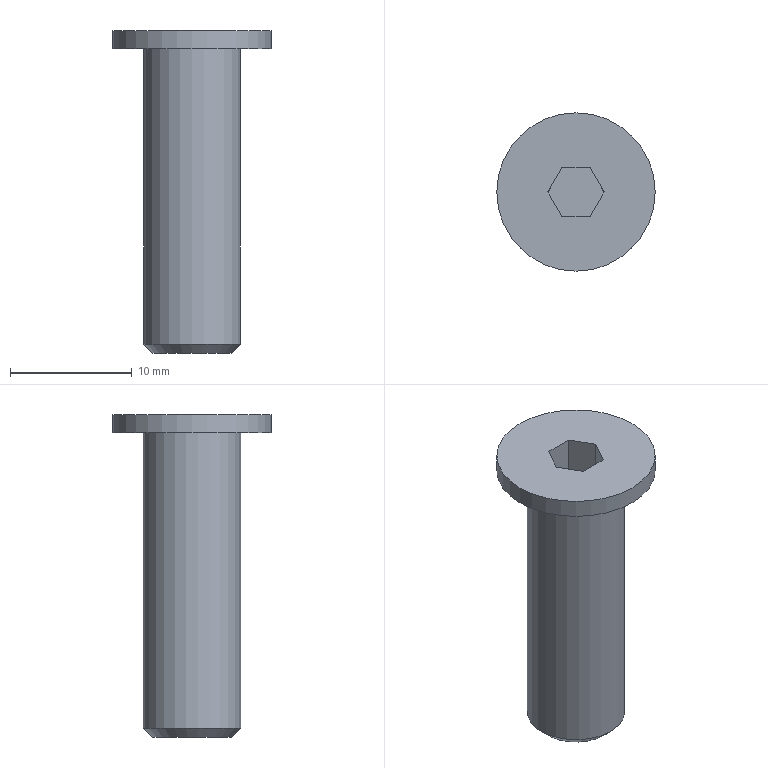Part | STEP file | 1 solid | 13 faces | box 13 x 13 x 26.5 mm | volume 1380 mm3 | plane 10 | cylinder 2 | cone 1 | commonest cylinder face diameters 8 x1 13 x1
STEP:
#1=CARTESIAN_POINT('',(0.,0.,0.));
#2=DIRECTION('',(0.,0.,1.));
#3=DIRECTION('',(1.,0.,0.));
#4=AXIS2_PLACEMENT_3D('',#1,#2,#3);
#5=CARTESIAN_POINT('',(0.,-6.5,26.5));
#6=VERTEX_POINT('',#5);
#7=CARTESIAN_POINT('',(0.,0.,26.5));
#8=DIRECTION('',(0.,0.,1.));
#9=DIRECTION('',(1.,0.,0.));
#10=AXIS2_PLACEMENT_3D('',#7,#8,#9);
#11=CIRCLE('',#10,6.5);
#12=CARTESIAN_POINT('',(0.,0.,25.75));
#13=DIRECTION('',(0.,0.,1.));
#14=DIRECTION('',(0.,1.,0.));
#15=AXIS2_PLACEMENT_3D('',#12,#13,#14);
#16=CYLINDRICAL_SURFACE('',#15,6.5);
#17=CARTESIAN_POINT('',(-1.571,0.75));
#18=DIRECTION('',(1.,0.));
#19=VECTOR('',#18,1.);
#20=LINE('',#17,#19);
#21=(GEOMETRIC_REPRESENTATION_CONTEXT(2)PARAMETRIC_REPRESENTATION_CONTEXT()REPRESENTATION_CONTEXT('',''));
#22=DEFINITIONAL_REPRESENTATION('',(#20),#21);
#23=PCURVE('',#16,#22);
#24=CARTESIAN_POINT('',(0.,3.25,26.5));
#25=DIRECTION('',(0.,0.,-1.));
#26=DIRECTION('',(-1.,0.,0.));
#27=AXIS2_PLACEMENT_3D('',#24,#25,#26);
#28=PLANE('',#27);
#29=CARTESIAN_POINT('',(-6.5,-3.25));
#30=CARTESIAN_POINT('',(-6.5,8.008));
#31=CARTESIAN_POINT('',(3.25,2.379));
#32=CARTESIAN_POINT('',(13.,-3.25));
#33=CARTESIAN_POINT('',(3.25,-8.879));
#34=CARTESIAN_POINT('',(-6.5,-14.508));
#35=CARTESIAN_POINT('',(-6.5,-3.25));
#36=(BOUNDED_CURVE()B_SPLINE_CURVE(2,(#29,#30,#31,#32,#33,#34,#35),.UNSPECIFIED.,.T.,.F.)B_SPLINE_CURVE_WITH_KNOTS((1,2,2,2,2,1),(-2.094,0.,2.094,4.189,6.283,8.378),.UNSPECIFIED.)CURVE()GEOMETRIC_REPRESENTATION_ITEM()RATIONAL_B_SPLINE_CURVE((1.,0.5,1.,0.5,1.,0.5,1.))REPRESENTATION_ITEM(''));
#37=(GEOMETRIC_REPRESENTATION_CONTEXT(2)PARAMETRIC_REPRESENTATION_CONTEXT()REPRESENTATION_CONTEXT('',''));
#38=DEFINITIONAL_REPRESENTATION('',(#36),#37);
#39=PCURVE('',#28,#38);
#40=SURFACE_CURVE('',#11,(#23,#39),.PCURVE_S1.);
#41=EDGE_CURVE('',#6,#6,#40,.T.);
#42=ORIENTED_EDGE('',*,*,#41,.F.);
#43=CARTESIAN_POINT('',(0.,-6.5,25.));
#44=VERTEX_POINT('',#43);
#45=CARTESIAN_POINT('',(0.,-6.5,25.));
#46=CARTESIAN_POINT('',(0.,-6.5,26.5));
#47=B_SPLINE_CURVE_WITH_KNOTS('',1,(#45,#46),.UNSPECIFIED.,.F.,.F.,(2,2),(-0.75,0.75),.PIECEWISE_BEZIER_KNOTS.);
#48=CARTESIAN_POINT('',(3.142,0.));
#49=DIRECTION('',(0.,1.));
#50=VECTOR('',#49,1.);
#51=LINE('',#48,#50);
#52=(GEOMETRIC_REPRESENTATION_CONTEXT(2)PARAMETRIC_REPRESENTATION_CONTEXT()REPRESENTATION_CONTEXT('',''));
#53=DEFINITIONAL_REPRESENTATION('',(#51),#52);
#54=PCURVE('',#16,#53);
#55=CARTESIAN_POINT('',(9.425,0.));
#56=DIRECTION('',(0.,1.));
#57=VECTOR('',#56,1.);
#58=LINE('',#55,#57);
#59=(GEOMETRIC_REPRESENTATION_CONTEXT(2)PARAMETRIC_REPRESENTATION_CONTEXT()REPRESENTATION_CONTEXT('',''));
#60=DEFINITIONAL_REPRESENTATION('',(#58),#59);
#61=PCURVE('',#16,#60);
#62=SEAM_CURVE('',#47,(#54,#61),.PCURVE_S1.);
#63=EDGE_CURVE('',#44,#6,#62,.T.);
#64=ORIENTED_EDGE('',*,*,#63,.F.);
#65=CARTESIAN_POINT('',(0.,0.,25.));
#66=DIRECTION('',(0.,0.,1.));
#67=DIRECTION('',(1.,0.,0.));
#68=AXIS2_PLACEMENT_3D('',#65,#66,#67);
#69=CIRCLE('',#68,6.5);
#70=CARTESIAN_POINT('',(-1.571,-0.75));
#71=DIRECTION('',(1.,0.));
#72=VECTOR('',#71,1.);
#73=LINE('',#70,#72);
#74=(GEOMETRIC_REPRESENTATION_CONTEXT(2)PARAMETRIC_REPRESENTATION_CONTEXT()REPRESENTATION_CONTEXT('',''));
#75=DEFINITIONAL_REPRESENTATION('',(#73),#74);
#76=PCURVE('',#16,#75);
#77=CARTESIAN_POINT('',(0.,5.25,25.));
#78=DIRECTION('',(0.,0.,-1.));
#79=DIRECTION('',(-1.,0.,0.));
#80=AXIS2_PLACEMENT_3D('',#77,#78,#79);
#81=PLANE('',#80);
#82=CARTESIAN_POINT('',(-6.5,-5.25));
#83=CARTESIAN_POINT('',(-6.5,6.008));
#84=CARTESIAN_POINT('',(3.25,0.3792));
#85=CARTESIAN_POINT('',(13.,-5.25));
#86=CARTESIAN_POINT('',(3.25,-10.879));
#87=CARTESIAN_POINT('',(-6.5,-16.508));
#88=CARTESIAN_POINT('',(-6.5,-5.25));
#89=(BOUNDED_CURVE()B_SPLINE_CURVE(2,(#82,#83,#84,#85,#86,#87,#88),.UNSPECIFIED.,.T.,.F.)B_SPLINE_CURVE_WITH_KNOTS((1,2,2,2,2,1),(-2.094,0.,2.094,4.189,6.283,8.378),.UNSPECIFIED.)CURVE()GEOMETRIC_REPRESENTATION_ITEM()RATIONAL_B_SPLINE_CURVE((1.,0.5,1.,0.5,1.,0.5,1.))REPRESENTATION_ITEM(''));
#90=(GEOMETRIC_REPRESENTATION_CONTEXT(2)PARAMETRIC_REPRESENTATION_CONTEXT()REPRESENTATION_CONTEXT('',''));
#91=DEFINITIONAL_REPRESENTATION('',(#89),#90);
#92=PCURVE('',#81,#91);
#93=SURFACE_CURVE('',#69,(#76,#92),.PCURVE_S1.);
#94=EDGE_CURVE('',#44,#44,#93,.T.);
#95=ORIENTED_EDGE('',*,*,#94,.T.);
#96=ORIENTED_EDGE('',*,*,#63,.T.);
#97=EDGE_LOOP('',(#42,#64,#95,#96));
#98=FACE_BOUND('',#97,.T.);
#99=ADVANCED_FACE('',(#98),#16,.T.);
#100=ORIENTED_EDGE('',*,*,#41,.T.);
#101=EDGE_LOOP('',(#100));
#102=FACE_BOUND('',#101,.T.);
#103=CARTESIAN_POINT('',(-2.309,0.,26.5));
#104=VERTEX_POINT('',#103);
#105=CARTESIAN_POINT('',(-1.155,2.,26.5));
#106=VERTEX_POINT('',#105);
#107=CARTESIAN_POINT('',(-2.309,0.,26.5));
#108=DIRECTION('',(0.5,0.866,0.));
#109=VECTOR('',#108,1.);
#110=LINE('',#107,#109);
#111=CARTESIAN_POINT('',(2.309,-3.25));
#112=DIRECTION('',(-0.5,0.866));
#113=VECTOR('',#112,1.);
#114=LINE('',#111,#113);
#115=(GEOMETRIC_REPRESENTATION_CONTEXT(2)PARAMETRIC_REPRESENTATION_CONTEXT()REPRESENTATION_CONTEXT('',''));
#116=DEFINITIONAL_REPRESENTATION('',(#114),#115);
#117=PCURVE('',#28,#116);
#118=CARTESIAN_POINT('',(-1.155,2.,26.5));
#119=DIRECTION('',(-0.866,0.5,0.));
#120=DIRECTION('',(0.,0.,1.));
#121=AXIS2_PLACEMENT_3D('',#118,#119,#120);
#122=PLANE('',#121);
#123=CARTESIAN_POINT('',(0.,-2.309));
#124=DIRECTION('',(0.,1.));
#125=VECTOR('',#124,1.);
#126=LINE('',#123,#125);
#127=(GEOMETRIC_REPRESENTATION_CONTEXT(2)PARAMETRIC_REPRESENTATION_CONTEXT()REPRESENTATION_CONTEXT('',''));
#128=DEFINITIONAL_REPRESENTATION('',(#126),#127);
#129=PCURVE('',#122,#128);
#130=SURFACE_CURVE('',#110,(#117,#129),.PCURVE_S1.);
#131=EDGE_CURVE('',#104,#106,#130,.T.);
#132=ORIENTED_EDGE('',*,*,#131,.T.);
#133=CARTESIAN_POINT('',(1.155,2.,26.5));
#134=VERTEX_POINT('',#133);
#135=CARTESIAN_POINT('',(-1.155,2.,26.5));
#136=DIRECTION('',(1.,0.,0.));
#137=VECTOR('',#136,1.);
#138=LINE('',#135,#137);
#139=CARTESIAN_POINT('',(1.155,-1.25));
#140=DIRECTION('',(-1.,0.));
#141=VECTOR('',#140,1.);
#142=LINE('',#139,#141);
#143=(GEOMETRIC_REPRESENTATION_CONTEXT(2)PARAMETRIC_REPRESENTATION_CONTEXT()REPRESENTATION_CONTEXT('',''));
#144=DEFINITIONAL_REPRESENTATION('',(#142),#143);
#145=PCURVE('',#28,#144);
#146=CARTESIAN_POINT('',(1.155,2.,26.5));
#147=DIRECTION('',(0.,1.,0.));
#148=DIRECTION('',(0.,0.,1.));
#149=AXIS2_PLACEMENT_3D('',#146,#147,#148);
#150=PLANE('',#149);
#151=CARTESIAN_POINT('',(0.,-2.309));
#152=DIRECTION('',(0.,1.));
#153=VECTOR('',#152,1.);
#154=LINE('',#151,#153);
#155=(GEOMETRIC_REPRESENTATION_CONTEXT(2)PARAMETRIC_REPRESENTATION_CONTEXT()REPRESENTATION_CONTEXT('',''));
#156=DEFINITIONAL_REPRESENTATION('',(#154),#155);
#157=PCURVE('',#150,#156);
#158=SURFACE_CURVE('',#138,(#145,#157),.PCURVE_S1.);
#159=EDGE_CURVE('',#106,#134,#158,.T.);
#160=ORIENTED_EDGE('',*,*,#159,.T.);
#161=CARTESIAN_POINT('',(2.309,0.,26.5));
#162=VERTEX_POINT('',#161);
#163=CARTESIAN_POINT('',(1.155,2.,26.5));
#164=DIRECTION('',(0.5,-0.866,0.));
#165=VECTOR('',#164,1.);
#166=LINE('',#163,#165);
#167=CARTESIAN_POINT('',(-1.155,-1.25));
#168=DIRECTION('',(-0.5,-0.866));
#169=VECTOR('',#168,1.);
#170=LINE('',#167,#169);
#171=(GEOMETRIC_REPRESENTATION_CONTEXT(2)PARAMETRIC_REPRESENTATION_CONTEXT()REPRESENTATION_CONTEXT('',''));
#172=DEFINITIONAL_REPRESENTATION('',(#170),#171);
#173=PCURVE('',#28,#172);
#174=CARTESIAN_POINT('',(2.309,0.,26.5));
#175=DIRECTION('',(0.866,0.5,0.));
#176=DIRECTION('',(0.,0.,-1.));
#177=AXIS2_PLACEMENT_3D('',#174,#175,#176);
#178=PLANE('',#177);
#179=CARTESIAN_POINT('',(0.,2.309));
#180=DIRECTION('',(0.,-1.));
#181=VECTOR('',#180,1.);
#182=LINE('',#179,#181);
#183=(GEOMETRIC_REPRESENTATION_CONTEXT(2)PARAMETRIC_REPRESENTATION_CONTEXT()REPRESENTATION_CONTEXT('',''));
#184=DEFINITIONAL_REPRESENTATION('',(#182),#183);
#185=PCURVE('',#178,#184);
#186=SURFACE_CURVE('',#166,(#173,#185),.PCURVE_S1.);
#187=EDGE_CURVE('',#134,#162,#186,.T.);
#188=ORIENTED_EDGE('',*,*,#187,.T.);
#189=CARTESIAN_POINT('',(1.155,-2.,26.5));
#190=VERTEX_POINT('',#189);
#191=CARTESIAN_POINT('',(2.309,0.,26.5));
#192=DIRECTION('',(-0.5,-0.866,0.));
#193=VECTOR('',#192,1.);
#194=LINE('',#191,#193);
#195=CARTESIAN_POINT('',(-2.309,-3.25));
#196=DIRECTION('',(0.5,-0.866));
#197=VECTOR('',#196,1.);
#198=LINE('',#195,#197);
#199=(GEOMETRIC_REPRESENTATION_CONTEXT(2)PARAMETRIC_REPRESENTATION_CONTEXT()REPRESENTATION_CONTEXT('',''));
#200=DEFINITIONAL_REPRESENTATION('',(#198),#199);
#201=PCURVE('',#28,#200);
#202=CARTESIAN_POINT('',(1.155,-2.,26.5));
#203=DIRECTION('',(0.866,-0.5,0.));
#204=DIRECTION('',(0.,0.,-1.));
#205=AXIS2_PLACEMENT_3D('',#202,#203,#204);
#206=PLANE('',#205);
#207=CARTESIAN_POINT('',(0.,2.309));
#208=DIRECTION('',(0.,-1.));
#209=VECTOR('',#208,1.);
#210=LINE('',#207,#209);
#211=(GEOMETRIC_REPRESENTATION_CONTEXT(2)PARAMETRIC_REPRESENTATION_CONTEXT()REPRESENTATION_CONTEXT('',''));
#212=DEFINITIONAL_REPRESENTATION('',(#210),#211);
#213=PCURVE('',#206,#212);
#214=SURFACE_CURVE('',#194,(#201,#213),.PCURVE_S1.);
#215=EDGE_CURVE('',#162,#190,#214,.T.);
#216=ORIENTED_EDGE('',*,*,#215,.T.);
#217=CARTESIAN_POINT('',(-1.155,-2.,26.5));
#218=VERTEX_POINT('',#217);
#219=CARTESIAN_POINT('',(1.155,-2.,26.5));
#220=DIRECTION('',(-1.,0.,0.));
#221=VECTOR('',#220,1.);
#222=LINE('',#219,#221);
#223=CARTESIAN_POINT('',(-1.155,-5.25));
#224=DIRECTION('',(1.,0.));
#225=VECTOR('',#224,1.);
#226=LINE('',#223,#225);
#227=(GEOMETRIC_REPRESENTATION_CONTEXT(2)PARAMETRIC_REPRESENTATION_CONTEXT()REPRESENTATION_CONTEXT('',''));
#228=DEFINITIONAL_REPRESENTATION('',(#226),#227);
#229=PCURVE('',#28,#228);
#230=CARTESIAN_POINT('',(-1.155,-2.,26.5));
#231=DIRECTION('',(0.,-1.,0.));
#232=DIRECTION('',(0.,0.,-1.));
#233=AXIS2_PLACEMENT_3D('',#230,#231,#232);
#234=PLANE('',#233);
#235=CARTESIAN_POINT('',(0.,2.309));
#236=DIRECTION('',(0.,-1.));
#237=VECTOR('',#236,1.);
#238=LINE('',#235,#237);
#239=(GEOMETRIC_REPRESENTATION_CONTEXT(2)PARAMETRIC_REPRESENTATION_CONTEXT()REPRESENTATION_CONTEXT('',''));
#240=DEFINITIONAL_REPRESENTATION('',(#238),#239);
#241=PCURVE('',#234,#240);
#242=SURFACE_CURVE('',#222,(#229,#241),.PCURVE_S1.);
#243=EDGE_CURVE('',#190,#218,#242,.T.);
#244=ORIENTED_EDGE('',*,*,#243,.T.);
#245=CARTESIAN_POINT('',(-1.155,-2.,26.5));
#246=DIRECTION('',(-0.5,0.866,0.));
#247=VECTOR('',#246,1.);
#248=LINE('',#245,#247);
#249=CARTESIAN_POINT('',(1.155,-5.25));
#250=DIRECTION('',(0.5,0.866));
#251=VECTOR('',#250,1.);
#252=LINE('',#249,#251);
#253=(GEOMETRIC_REPRESENTATION_CONTEXT(2)PARAMETRIC_REPRESENTATION_CONTEXT()REPRESENTATION_CONTEXT('',''));
#254=DEFINITIONAL_REPRESENTATION('',(#252),#253);
#255=PCURVE('',#28,#254);
#256=CARTESIAN_POINT('',(-2.309,0.,26.5));
#257=DIRECTION('',(-0.866,-0.5,0.));
#258=DIRECTION('',(0.,0.,1.));
#259=AXIS2_PLACEMENT_3D('',#256,#257,#258);
#260=PLANE('',#259);
#261=CARTESIAN_POINT('',(0.,-2.309));
#262=DIRECTION('',(0.,1.));
#263=VECTOR('',#262,1.);
#264=LINE('',#261,#263);
#265=(GEOMETRIC_REPRESENTATION_CONTEXT(2)PARAMETRIC_REPRESENTATION_CONTEXT()REPRESENTATION_CONTEXT('',''));
#266=DEFINITIONAL_REPRESENTATION('',(#264),#265);
#267=PCURVE('',#260,#266);
#268=SURFACE_CURVE('',#248,(#255,#267),.PCURVE_S1.);
#269=EDGE_CURVE('',#218,#104,#268,.T.);
#270=ORIENTED_EDGE('',*,*,#269,.T.);
#271=EDGE_LOOP('',(#132,#160,#188,#216,#244,#270));
#272=FACE_BOUND('',#271,.T.);
#273=ADVANCED_FACE('',(#102,#272),#28,.F.);
#274=ORIENTED_EDGE('',*,*,#94,.F.);
#275=EDGE_LOOP('',(#274));
#276=FACE_BOUND('',#275,.T.);
#277=CARTESIAN_POINT('',(0.,-4.,25.));
#278=VERTEX_POINT('',#277);
#279=CARTESIAN_POINT('',(0.,0.,25.));
#280=DIRECTION('',(0.,0.,-1.));
#281=DIRECTION('',(1.,0.,0.));
#282=AXIS2_PLACEMENT_3D('',#279,#280,#281);
#283=CIRCLE('',#282,4.);
#284=CARTESIAN_POINT('',(0.,-5.25));
#285=DIRECTION('',(-1.,0.));
#286=AXIS2_PLACEMENT_2D('',#284,#285);
#287=CIRCLE('',#286,4.);
#288=(GEOMETRIC_REPRESENTATION_CONTEXT(2)PARAMETRIC_REPRESENTATION_CONTEXT()REPRESENTATION_CONTEXT('',''));
#289=DEFINITIONAL_REPRESENTATION('',(#287),#288);
#290=PCURVE('',#81,#289);
#291=CARTESIAN_POINT('',(0.,0.,12.883));
#292=DIRECTION('',(0.,0.,1.));
#293=DIRECTION('',(0.,1.,0.));
#294=AXIS2_PLACEMENT_3D('',#291,#292,#293);
#295=CYLINDRICAL_SURFACE('',#294,4.);
#296=CARTESIAN_POINT('',(10.996,12.117));
#297=DIRECTION('',(-1.,0.));
#298=VECTOR('',#297,1.);
#299=LINE('',#296,#298);
#300=(GEOMETRIC_REPRESENTATION_CONTEXT(2)PARAMETRIC_REPRESENTATION_CONTEXT()REPRESENTATION_CONTEXT('',''));
#301=DEFINITIONAL_REPRESENTATION('',(#299),#300);
#302=PCURVE('',#295,#301);
#303=SURFACE_CURVE('',#283,(#290,#302),.PCURVE_S1.);
#304=EDGE_CURVE('',#278,#278,#303,.T.);
#305=ORIENTED_EDGE('',*,*,#304,.F.);
#306=EDGE_LOOP('',(#305));
#307=FACE_BOUND('',#306,.T.);
#308=ADVANCED_FACE('',(#276,#307),#81,.T.);
#309=CARTESIAN_POINT('',(-2.309,0.,21.5));
#310=VERTEX_POINT('',#309);
#311=CARTESIAN_POINT('',(-2.309,0.,26.5));
#312=DIRECTION('',(0.,0.,-1.));
#313=VECTOR('',#312,1.);
#314=LINE('',#311,#313);
#315=CARTESIAN_POINT('',(0.,-2.309));
#316=DIRECTION('',(-1.,0.));
#317=VECTOR('',#316,1.);
#318=LINE('',#315,#317);
#319=(GEOMETRIC_REPRESENTATION_CONTEXT(2)PARAMETRIC_REPRESENTATION_CONTEXT()REPRESENTATION_CONTEXT('',''));
#320=DEFINITIONAL_REPRESENTATION('',(#318),#319);
#321=PCURVE('',#122,#320);
#322=CARTESIAN_POINT('',(0.,0.));
#323=DIRECTION('',(-1.,0.));
#324=VECTOR('',#323,1.);
#325=LINE('',#322,#324);
#326=(GEOMETRIC_REPRESENTATION_CONTEXT(2)PARAMETRIC_REPRESENTATION_CONTEXT()REPRESENTATION_CONTEXT('',''));
#327=DEFINITIONAL_REPRESENTATION('',(#325),#326);
#328=PCURVE('',#260,#327);
#329=SURFACE_CURVE('',#314,(#321,#328),.PCURVE_S1.);
#330=EDGE_CURVE('',#104,#310,#329,.T.);
#331=ORIENTED_EDGE('',*,*,#330,.T.);
#332=CARTESIAN_POINT('',(-1.155,2.,21.5));
#333=VERTEX_POINT('',#332);
#334=CARTESIAN_POINT('',(-1.155,2.,21.5));
#335=DIRECTION('',(-0.5,-0.866,0.));
#336=VECTOR('',#335,1.);
#337=LINE('',#334,#336);
#338=CARTESIAN_POINT('',(-5.,0.));
#339=DIRECTION('',(0.,-1.));
#340=VECTOR('',#339,1.);
#341=LINE('',#338,#340);
#342=(GEOMETRIC_REPRESENTATION_CONTEXT(2)PARAMETRIC_REPRESENTATION_CONTEXT()REPRESENTATION_CONTEXT('',''));
#343=DEFINITIONAL_REPRESENTATION('',(#341),#342);
#344=PCURVE('',#122,#343);
#345=CARTESIAN_POINT('',(0.,0.,21.5));
#346=DIRECTION('',(0.,0.,1.));
#347=DIRECTION('',(1.,0.,0.));
#348=AXIS2_PLACEMENT_3D('',#345,#346,#347);
#349=PLANE('',#348);
#350=CARTESIAN_POINT('',(-1.155,2.));
#351=DIRECTION('',(-0.5,-0.866));
#352=VECTOR('',#351,1.);
#353=LINE('',#350,#352);
#354=(GEOMETRIC_REPRESENTATION_CONTEXT(2)PARAMETRIC_REPRESENTATION_CONTEXT()REPRESENTATION_CONTEXT('',''));
#355=DEFINITIONAL_REPRESENTATION('',(#353),#354);
#356=PCURVE('',#349,#355);
#357=SURFACE_CURVE('',#337,(#344,#356),.PCURVE_S1.);
#358=EDGE_CURVE('',#333,#310,#357,.T.);
#359=ORIENTED_EDGE('',*,*,#358,.F.);
#360=CARTESIAN_POINT('',(-1.155,2.,26.5));
#361=DIRECTION('',(0.,0.,-1.));
#362=VECTOR('',#361,1.);
#363=LINE('',#360,#362);
#364=CARTESIAN_POINT('',(0.,0.));
#365=DIRECTION('',(-1.,0.));
#366=VECTOR('',#365,1.);
#367=LINE('',#364,#366);
#368=(GEOMETRIC_REPRESENTATION_CONTEXT(2)PARAMETRIC_REPRESENTATION_CONTEXT()REPRESENTATION_CONTEXT('',''));
#369=DEFINITIONAL_REPRESENTATION('',(#367),#368);
#370=PCURVE('',#122,#369);
#371=CARTESIAN_POINT('',(0.,-2.309));
#372=DIRECTION('',(-1.,0.));
#373=VECTOR('',#372,1.);
#374=LINE('',#371,#373);
#375=(GEOMETRIC_REPRESENTATION_CONTEXT(2)PARAMETRIC_REPRESENTATION_CONTEXT()REPRESENTATION_CONTEXT('',''));
#376=DEFINITIONAL_REPRESENTATION('',(#374),#375);
#377=PCURVE('',#150,#376);
#378=SURFACE_CURVE('',#363,(#370,#377),.PCURVE_S1.);
#379=EDGE_CURVE('',#106,#333,#378,.T.);
#380=ORIENTED_EDGE('',*,*,#379,.F.);
#381=ORIENTED_EDGE('',*,*,#131,.F.);
#382=EDGE_LOOP('',(#331,#359,#380,#381));
#383=FACE_BOUND('',#382,.T.);
#384=ADVANCED_FACE('',(#383),#122,.F.);
#385=ORIENTED_EDGE('',*,*,#379,.T.);
#386=CARTESIAN_POINT('',(1.155,2.,21.5));
#387=VERTEX_POINT('',#386);
#388=CARTESIAN_POINT('',(1.155,2.,21.5));
#389=DIRECTION('',(-1.,0.,0.));
#390=VECTOR('',#389,1.);
#391=LINE('',#388,#390);
#392=CARTESIAN_POINT('',(-5.,0.));
#393=DIRECTION('',(0.,-1.));
#394=VECTOR('',#393,1.);
#395=LINE('',#392,#394);
#396=(GEOMETRIC_REPRESENTATION_CONTEXT(2)PARAMETRIC_REPRESENTATION_CONTEXT()REPRESENTATION_CONTEXT('',''));
#397=DEFINITIONAL_REPRESENTATION('',(#395),#396);
#398=PCURVE('',#150,#397);
#399=CARTESIAN_POINT('',(1.155,2.));
#400=DIRECTION('',(-1.,0.));
#401=VECTOR('',#400,1.);
#402=LINE('',#399,#401);
#403=(GEOMETRIC_REPRESENTATION_CONTEXT(2)PARAMETRIC_REPRESENTATION_CONTEXT()REPRESENTATION_CONTEXT('',''));
#404=DEFINITIONAL_REPRESENTATION('',(#402),#403);
#405=PCURVE('',#349,#404);
#406=SURFACE_CURVE('',#391,(#398,#405),.PCURVE_S1.);
#407=EDGE_CURVE('',#387,#333,#406,.T.);
#408=ORIENTED_EDGE('',*,*,#407,.F.);
#409=CARTESIAN_POINT('',(1.155,2.,26.5));
#410=DIRECTION('',(0.,0.,-1.));
#411=VECTOR('',#410,1.);
#412=LINE('',#409,#411);
#413=CARTESIAN_POINT('',(0.,0.));
#414=DIRECTION('',(-1.,0.));
#415=VECTOR('',#414,1.);
#416=LINE('',#413,#415);
#417=(GEOMETRIC_REPRESENTATION_CONTEXT(2)PARAMETRIC_REPRESENTATION_CONTEXT()REPRESENTATION_CONTEXT('',''));
#418=DEFINITIONAL_REPRESENTATION('',(#416),#417);
#419=PCURVE('',#150,#418);
#420=CARTESIAN_POINT('',(0.,2.309));
#421=DIRECTION('',(1.,0.));
#422=VECTOR('',#421,1.);
#423=LINE('',#420,#422);
#424=(GEOMETRIC_REPRESENTATION_CONTEXT(2)PARAMETRIC_REPRESENTATION_CONTEXT()REPRESENTATION_CONTEXT('',''));
#425=DEFINITIONAL_REPRESENTATION('',(#423),#424);
#426=PCURVE('',#178,#425);
#427=SURFACE_CURVE('',#412,(#419,#426),.PCURVE_S1.);
#428=EDGE_CURVE('',#134,#387,#427,.T.);
#429=ORIENTED_EDGE('',*,*,#428,.F.);
#430=ORIENTED_EDGE('',*,*,#159,.F.);
#431=EDGE_LOOP('',(#385,#408,#429,#430));
#432=FACE_BOUND('',#431,.T.);
#433=ADVANCED_FACE('',(#432),#150,.F.);
#434=ORIENTED_EDGE('',*,*,#428,.T.);
#435=CARTESIAN_POINT('',(2.309,0.,21.5));
#436=VERTEX_POINT('',#435);
#437=CARTESIAN_POINT('',(2.309,0.,21.5));
#438=DIRECTION('',(-0.5,0.866,0.));
#439=VECTOR('',#438,1.);
#440=LINE('',#437,#439);
#441=CARTESIAN_POINT('',(5.,0.));
#442=DIRECTION('',(0.,1.));
#443=VECTOR('',#442,1.);
#444=LINE('',#441,#443);
#445=(GEOMETRIC_REPRESENTATION_CONTEXT(2)PARAMETRIC_REPRESENTATION_CONTEXT()REPRESENTATION_CONTEXT('',''));
#446=DEFINITIONAL_REPRESENTATION('',(#444),#445);
#447=PCURVE('',#178,#446);
#448=CARTESIAN_POINT('',(2.309,0.));
#449=DIRECTION('',(-0.5,0.866));
#450=VECTOR('',#449,1.);
#451=LINE('',#448,#450);
#452=(GEOMETRIC_REPRESENTATION_CONTEXT(2)PARAMETRIC_REPRESENTATION_CONTEXT()REPRESENTATION_CONTEXT('',''));
#453=DEFINITIONAL_REPRESENTATION('',(#451),#452);
#454=PCURVE('',#349,#453);
#455=SURFACE_CURVE('',#440,(#447,#454),.PCURVE_S1.);
#456=EDGE_CURVE('',#436,#387,#455,.T.);
#457=ORIENTED_EDGE('',*,*,#456,.F.);
#458=CARTESIAN_POINT('',(2.309,0.,26.5));
#459=DIRECTION('',(0.,0.,-1.));
#460=VECTOR('',#459,1.);
#461=LINE('',#458,#460);
#462=CARTESIAN_POINT('',(0.,0.));
#463=DIRECTION('',(1.,0.));
#464=VECTOR('',#463,1.);
#465=LINE('',#462,#464);
#466=(GEOMETRIC_REPRESENTATION_CONTEXT(2)PARAMETRIC_REPRESENTATION_CONTEXT()REPRESENTATION_CONTEXT('',''));
#467=DEFINITIONAL_REPRESENTATION('',(#465),#466);
#468=PCURVE('',#178,#467);
#469=CARTESIAN_POINT('',(0.,2.309));
#470=DIRECTION('',(1.,0.));
#471=VECTOR('',#470,1.);
#472=LINE('',#469,#471);
#473=(GEOMETRIC_REPRESENTATION_CONTEXT(2)PARAMETRIC_REPRESENTATION_CONTEXT()REPRESENTATION_CONTEXT('',''));
#474=DEFINITIONAL_REPRESENTATION('',(#472),#473);
#475=PCURVE('',#206,#474);
#476=SURFACE_CURVE('',#461,(#468,#475),.PCURVE_S1.);
#477=EDGE_CURVE('',#162,#436,#476,.T.);
#478=ORIENTED_EDGE('',*,*,#477,.F.);
#479=ORIENTED_EDGE('',*,*,#187,.F.);
#480=EDGE_LOOP('',(#434,#457,#478,#479));
#481=FACE_BOUND('',#480,.T.);
#482=ADVANCED_FACE('',(#481),#178,.F.);
#483=ORIENTED_EDGE('',*,*,#477,.T.);
#484=CARTESIAN_POINT('',(1.155,-2.,21.5));
#485=VERTEX_POINT('',#484);
#486=CARTESIAN_POINT('',(1.155,-2.,21.5));
#487=DIRECTION('',(0.5,0.866,0.));
#488=VECTOR('',#487,1.);
#489=LINE('',#486,#488);
#490=CARTESIAN_POINT('',(5.,0.));
#491=DIRECTION('',(0.,1.));
#492=VECTOR('',#491,1.);
#493=LINE('',#490,#492);
#494=(GEOMETRIC_REPRESENTATION_CONTEXT(2)PARAMETRIC_REPRESENTATION_CONTEXT()REPRESENTATION_CONTEXT('',''));
#495=DEFINITIONAL_REPRESENTATION('',(#493),#494);
#496=PCURVE('',#206,#495);
#497=CARTESIAN_POINT('',(1.155,-2.));
#498=DIRECTION('',(0.5,0.866));
#499=VECTOR('',#498,1.);
#500=LINE('',#497,#499);
#501=(GEOMETRIC_REPRESENTATION_CONTEXT(2)PARAMETRIC_REPRESENTATION_CONTEXT()REPRESENTATION_CONTEXT('',''));
#502=DEFINITIONAL_REPRESENTATION('',(#500),#501);
#503=PCURVE('',#349,#502);
#504=SURFACE_CURVE('',#489,(#496,#503),.PCURVE_S1.);
#505=EDGE_CURVE('',#485,#436,#504,.T.);
#506=ORIENTED_EDGE('',*,*,#505,.F.);
#507=CARTESIAN_POINT('',(1.155,-2.,26.5));
#508=DIRECTION('',(0.,0.,-1.));
#509=VECTOR('',#508,1.);
#510=LINE('',#507,#509);
#511=CARTESIAN_POINT('',(0.,0.));
#512=DIRECTION('',(1.,0.));
#513=VECTOR('',#512,1.);
#514=LINE('',#511,#513);
#515=(GEOMETRIC_REPRESENTATION_CONTEXT(2)PARAMETRIC_REPRESENTATION_CONTEXT()REPRESENTATION_CONTEXT('',''));
#516=DEFINITIONAL_REPRESENTATION('',(#514),#515);
#517=PCURVE('',#206,#516);
#518=CARTESIAN_POINT('',(0.,2.309));
#519=DIRECTION('',(1.,0.));
#520=VECTOR('',#519,1.);
#521=LINE('',#518,#520);
#522=(GEOMETRIC_REPRESENTATION_CONTEXT(2)PARAMETRIC_REPRESENTATION_CONTEXT()REPRESENTATION_CONTEXT('',''));
#523=DEFINITIONAL_REPRESENTATION('',(#521),#522);
#524=PCURVE('',#234,#523);
#525=SURFACE_CURVE('',#510,(#517,#524),.PCURVE_S1.);
#526=EDGE_CURVE('',#190,#485,#525,.T.);
#527=ORIENTED_EDGE('',*,*,#526,.F.);
#528=ORIENTED_EDGE('',*,*,#215,.F.);
#529=EDGE_LOOP('',(#483,#506,#527,#528));
#530=FACE_BOUND('',#529,.T.);
#531=ADVANCED_FACE('',(#530),#206,.F.);
#532=ORIENTED_EDGE('',*,*,#526,.T.);
#533=CARTESIAN_POINT('',(-1.155,-2.,21.5));
#534=VERTEX_POINT('',#533);
#535=CARTESIAN_POINT('',(-1.155,-2.,21.5));
#536=DIRECTION('',(1.,0.,0.));
#537=VECTOR('',#536,1.);
#538=LINE('',#535,#537);
#539=CARTESIAN_POINT('',(5.,0.));
#540=DIRECTION('',(0.,1.));
#541=VECTOR('',#540,1.);
#542=LINE('',#539,#541);
#543=(GEOMETRIC_REPRESENTATION_CONTEXT(2)PARAMETRIC_REPRESENTATION_CONTEXT()REPRESENTATION_CONTEXT('',''));
#544=DEFINITIONAL_REPRESENTATION('',(#542),#543);
#545=PCURVE('',#234,#544);
#546=CARTESIAN_POINT('',(-1.155,-2.));
#547=DIRECTION('',(1.,0.));
#548=VECTOR('',#547,1.);
#549=LINE('',#546,#548);
#550=(GEOMETRIC_REPRESENTATION_CONTEXT(2)PARAMETRIC_REPRESENTATION_CONTEXT()REPRESENTATION_CONTEXT('',''));
#551=DEFINITIONAL_REPRESENTATION('',(#549),#550);
#552=PCURVE('',#349,#551);
#553=SURFACE_CURVE('',#538,(#545,#552),.PCURVE_S1.);
#554=EDGE_CURVE('',#534,#485,#553,.T.);
#555=ORIENTED_EDGE('',*,*,#554,.F.);
#556=CARTESIAN_POINT('',(-1.155,-2.,26.5));
#557=DIRECTION('',(0.,0.,-1.));
#558=VECTOR('',#557,1.);
#559=LINE('',#556,#558);
#560=CARTESIAN_POINT('',(0.,0.));
#561=DIRECTION('',(1.,0.));
#562=VECTOR('',#561,1.);
#563=LINE('',#560,#562);
#564=(GEOMETRIC_REPRESENTATION_CONTEXT(2)PARAMETRIC_REPRESENTATION_CONTEXT()REPRESENTATION_CONTEXT('',''));
#565=DEFINITIONAL_REPRESENTATION('',(#563),#564);
#566=PCURVE('',#234,#565);
#567=CARTESIAN_POINT('',(0.,-2.309));
#568=DIRECTION('',(-1.,0.));
#569=VECTOR('',#568,1.);
#570=LINE('',#567,#569);
#571=(GEOMETRIC_REPRESENTATION_CONTEXT(2)PARAMETRIC_REPRESENTATION_CONTEXT()REPRESENTATION_CONTEXT('',''));
#572=DEFINITIONAL_REPRESENTATION('',(#570),#571);
#573=PCURVE('',#260,#572);
#574=SURFACE_CURVE('',#559,(#566,#573),.PCURVE_S1.);
#575=EDGE_CURVE('',#218,#534,#574,.T.);
#576=ORIENTED_EDGE('',*,*,#575,.F.);
#577=ORIENTED_EDGE('',*,*,#243,.F.);
#578=EDGE_LOOP('',(#532,#555,#576,#577));
#579=FACE_BOUND('',#578,.T.);
#580=ADVANCED_FACE('',(#579),#234,.F.);
#581=ORIENTED_EDGE('',*,*,#575,.T.);
#582=CARTESIAN_POINT('',(-2.309,0.,21.5));
#583=DIRECTION('',(0.5,-0.866,0.));
#584=VECTOR('',#583,1.);
#585=LINE('',#582,#584);
#586=CARTESIAN_POINT('',(-5.,0.));
#587=DIRECTION('',(0.,-1.));
#588=VECTOR('',#587,1.);
#589=LINE('',#586,#588);
#590=(GEOMETRIC_REPRESENTATION_CONTEXT(2)PARAMETRIC_REPRESENTATION_CONTEXT()REPRESENTATION_CONTEXT('',''));
#591=DEFINITIONAL_REPRESENTATION('',(#589),#590);
#592=PCURVE('',#260,#591);
#593=CARTESIAN_POINT('',(-2.309,0.));
#594=DIRECTION('',(0.5,-0.866));
#595=VECTOR('',#594,1.);
#596=LINE('',#593,#595);
#597=(GEOMETRIC_REPRESENTATION_CONTEXT(2)PARAMETRIC_REPRESENTATION_CONTEXT()REPRESENTATION_CONTEXT('',''));
#598=DEFINITIONAL_REPRESENTATION('',(#596),#597);
#599=PCURVE('',#349,#598);
#600=SURFACE_CURVE('',#585,(#592,#599),.PCURVE_S1.);
#601=EDGE_CURVE('',#310,#534,#600,.T.);
#602=ORIENTED_EDGE('',*,*,#601,.F.);
#603=ORIENTED_EDGE('',*,*,#330,.F.);
#604=ORIENTED_EDGE('',*,*,#269,.F.);
#605=EDGE_LOOP('',(#581,#602,#603,#604));
#606=FACE_BOUND('',#605,.T.);
#607=ADVANCED_FACE('',(#606),#260,.F.);
#608=ORIENTED_EDGE('',*,*,#304,.T.);
#609=CARTESIAN_POINT('',(0.,-4.,0.767));
#610=VERTEX_POINT('',#609);
#611=CARTESIAN_POINT('',(0.,-4.,0.767));
#612=CARTESIAN_POINT('',(0.,-4.,25.));
#613=B_SPLINE_CURVE_WITH_KNOTS('',1,(#611,#612),.UNSPECIFIED.,.F.,.F.,(2,2),(-12.116,12.117),.PIECEWISE_BEZIER_KNOTS.);
#614=CARTESIAN_POINT('',(3.142,0.));
#615=DIRECTION('',(0.,1.));
#616=VECTOR('',#615,1.);
#617=LINE('',#614,#616);
#618=(GEOMETRIC_REPRESENTATION_CONTEXT(2)PARAMETRIC_REPRESENTATION_CONTEXT()REPRESENTATION_CONTEXT('',''));
#619=DEFINITIONAL_REPRESENTATION('',(#617),#618);
#620=PCURVE('',#295,#619);
#621=CARTESIAN_POINT('',(9.425,0.));
#622=DIRECTION('',(0.,1.));
#623=VECTOR('',#622,1.);
#624=LINE('',#621,#623);
#625=(GEOMETRIC_REPRESENTATION_CONTEXT(2)PARAMETRIC_REPRESENTATION_CONTEXT()REPRESENTATION_CONTEXT('',''));
#626=DEFINITIONAL_REPRESENTATION('',(#624),#625);
#627=PCURVE('',#295,#626);
#628=SEAM_CURVE('',#613,(#620,#627),.PCURVE_S1.);
#629=EDGE_CURVE('',#610,#278,#628,.T.);
#630=ORIENTED_EDGE('',*,*,#629,.F.);
#631=CARTESIAN_POINT('',(0.,0.,0.767));
#632=DIRECTION('',(0.,0.,1.));
#633=DIRECTION('',(1.,0.,0.));
#634=AXIS2_PLACEMENT_3D('',#631,#632,#633);
#635=CIRCLE('',#634,4.);
#636=CARTESIAN_POINT('',(-1.571,-12.116));
#637=DIRECTION('',(1.,0.));
#638=VECTOR('',#637,1.);
#639=LINE('',#636,#638);
#640=(GEOMETRIC_REPRESENTATION_CONTEXT(2)PARAMETRIC_REPRESENTATION_CONTEXT()REPRESENTATION_CONTEXT('',''));
#641=DEFINITIONAL_REPRESENTATION('',(#639),#640);
#642=PCURVE('',#295,#641);
#643=CARTESIAN_POINT('',(0.,0.,0.767));
#644=DIRECTION('',(0.,0.,1.));
#645=DIRECTION('',(0.,1.,0.));
#646=AXIS2_PLACEMENT_3D('',#643,#644,#645);
#647=CONICAL_SURFACE('',#646,4.,0.7854);
#648=CARTESIAN_POINT('',(-1.571,0.));
#649=DIRECTION('',(1.,0.));
#650=VECTOR('',#649,1.);
#651=LINE('',#648,#650);
#652=(GEOMETRIC_REPRESENTATION_CONTEXT(2)PARAMETRIC_REPRESENTATION_CONTEXT()REPRESENTATION_CONTEXT('',''));
#653=DEFINITIONAL_REPRESENTATION('',(#651),#652);
#654=PCURVE('',#647,#653);
#655=SURFACE_CURVE('',#635,(#642,#654),.PCURVE_S1.);
#656=EDGE_CURVE('',#610,#610,#655,.T.);
#657=ORIENTED_EDGE('',*,*,#656,.T.);
#658=ORIENTED_EDGE('',*,*,#629,.T.);
#659=EDGE_LOOP('',(#608,#630,#657,#658));
#660=FACE_BOUND('',#659,.T.);
#661=ADVANCED_FACE('',(#660),#295,.T.);
#662=ORIENTED_EDGE('',*,*,#554,.T.);
#663=ORIENTED_EDGE('',*,*,#505,.T.);
#664=ORIENTED_EDGE('',*,*,#456,.T.);
#665=ORIENTED_EDGE('',*,*,#407,.T.);
#666=ORIENTED_EDGE('',*,*,#358,.T.);
#667=ORIENTED_EDGE('',*,*,#601,.T.);
#668=EDGE_LOOP('',(#662,#663,#664,#665,#666,#667));
#669=FACE_BOUND('',#668,.T.);
#670=ADVANCED_FACE('',(#669),#349,.T.);
#671=ORIENTED_EDGE('',*,*,#656,.F.);
#672=CARTESIAN_POINT('',(0.,-3.233,0.));
#673=VERTEX_POINT('',#672);
#674=CARTESIAN_POINT('',(0.,-3.233,-0.000000001));
#675=CARTESIAN_POINT('',(0.,-4.,0.767));
#676=B_SPLINE_CURVE_WITH_KNOTS('',1,(#674,#675),.UNSPECIFIED.,.F.,.F.,(2,2),(-1.085,0.),.PIECEWISE_BEZIER_KNOTS.);
#677=CARTESIAN_POINT('',(3.142,0.));
#678=DIRECTION('',(0.,1.));
#679=VECTOR('',#678,1.);
#680=LINE('',#677,#679);
#681=(GEOMETRIC_REPRESENTATION_CONTEXT(2)PARAMETRIC_REPRESENTATION_CONTEXT()REPRESENTATION_CONTEXT('',''));
#682=DEFINITIONAL_REPRESENTATION('',(#680),#681);
#683=PCURVE('',#647,#682);
#684=CARTESIAN_POINT('',(9.425,0.));
#685=DIRECTION('',(0.,1.));
#686=VECTOR('',#685,1.);
#687=LINE('',#684,#686);
#688=(GEOMETRIC_REPRESENTATION_CONTEXT(2)PARAMETRIC_REPRESENTATION_CONTEXT()REPRESENTATION_CONTEXT('',''));
#689=DEFINITIONAL_REPRESENTATION('',(#687),#688);
#690=PCURVE('',#647,#689);
#691=SEAM_CURVE('',#676,(#683,#690),.PCURVE_S1.);
#692=EDGE_CURVE('',#673,#610,#691,.T.);
#693=ORIENTED_EDGE('',*,*,#692,.F.);
#694=CARTESIAN_POINT('',(0.,0.,0.));
#695=DIRECTION('',(0.,0.,1.));
#696=DIRECTION('',(1.,0.,0.));
#697=AXIS2_PLACEMENT_3D('',#694,#695,#696);
#698=CIRCLE('',#697,3.233);
#699=CARTESIAN_POINT('',(-1.571,-0.767));
#700=DIRECTION('',(1.,0.));
#701=VECTOR('',#700,1.);
#702=LINE('',#699,#701);
#703=(GEOMETRIC_REPRESENTATION_CONTEXT(2)PARAMETRIC_REPRESENTATION_CONTEXT()REPRESENTATION_CONTEXT('',''));
#704=DEFINITIONAL_REPRESENTATION('',(#702),#703);
#705=PCURVE('',#647,#704);
#706=CARTESIAN_POINT('',(0.,1.617,0.));
#707=DIRECTION('',(0.,0.,-1.));
#708=DIRECTION('',(-1.,0.,0.));
#709=AXIS2_PLACEMENT_3D('',#706,#707,#708);
#710=PLANE('',#709);
#711=CARTESIAN_POINT('',(-3.233,-1.617));
#712=CARTESIAN_POINT('',(-3.233,3.983));
#713=CARTESIAN_POINT('',(1.617,1.183));
#714=CARTESIAN_POINT('',(6.466,-1.617));
#715=CARTESIAN_POINT('',(1.617,-4.416));
#716=CARTESIAN_POINT('',(-3.233,-7.216));
#717=CARTESIAN_POINT('',(-3.233,-1.617));
#718=(BOUNDED_CURVE()B_SPLINE_CURVE(2,(#711,#712,#713,#714,#715,#716,#717),.UNSPECIFIED.,.T.,.F.)B_SPLINE_CURVE_WITH_KNOTS((1,2,2,2,2,1),(-2.094,0.,2.094,4.189,6.283,8.378),.UNSPECIFIED.)CURVE()GEOMETRIC_REPRESENTATION_ITEM()RATIONAL_B_SPLINE_CURVE((1.,0.5,1.,0.5,1.,0.5,1.))REPRESENTATION_ITEM(''));
#719=(GEOMETRIC_REPRESENTATION_CONTEXT(2)PARAMETRIC_REPRESENTATION_CONTEXT()REPRESENTATION_CONTEXT('',''));
#720=DEFINITIONAL_REPRESENTATION('',(#718),#719);
#721=PCURVE('',#710,#720);
#722=SURFACE_CURVE('',#698,(#705,#721),.PCURVE_S1.);
#723=EDGE_CURVE('',#673,#673,#722,.T.);
#724=ORIENTED_EDGE('',*,*,#723,.T.);
#725=ORIENTED_EDGE('',*,*,#692,.T.);
#726=EDGE_LOOP('',(#671,#693,#724,#725));
#727=FACE_BOUND('',#726,.T.);
#728=ADVANCED_FACE('',(#727),#647,.T.);
#729=ORIENTED_EDGE('',*,*,#723,.F.);
#730=EDGE_LOOP('',(#729));
#731=FACE_BOUND('',#730,.T.);
#732=ADVANCED_FACE('',(#731),#710,.T.);
#733=CLOSED_SHELL('',(#99,#273,#308,#384,#433,#482,#531,#580,#607,#661,#670,#728,#732));
#734=MANIFOLD_SOLID_BREP('',#733);
#735=(LENGTH_UNIT()NAMED_UNIT(*)SI_UNIT(.MILLI.,.METRE.));
#736=UNCERTAINTY_MEASURE_WITH_UNIT(LENGTH_MEASURE(0.000002),#735,'','');
#737=(NAMED_UNIT(*)PLANE_ANGLE_UNIT()SI_UNIT($,.RADIAN.));
#738=(NAMED_UNIT(*)SI_UNIT($,.STERADIAN.)SOLID_ANGLE_UNIT());
#739=(GEOMETRIC_REPRESENTATION_CONTEXT(3)GLOBAL_UNCERTAINTY_ASSIGNED_CONTEXT((#736))GLOBAL_UNIT_ASSIGNED_CONTEXT((#735,#737,#738))REPRESENTATION_CONTEXT('',''));
#740=ADVANCED_BREP_SHAPE_REPRESENTATION('',(#4,#734),#739);